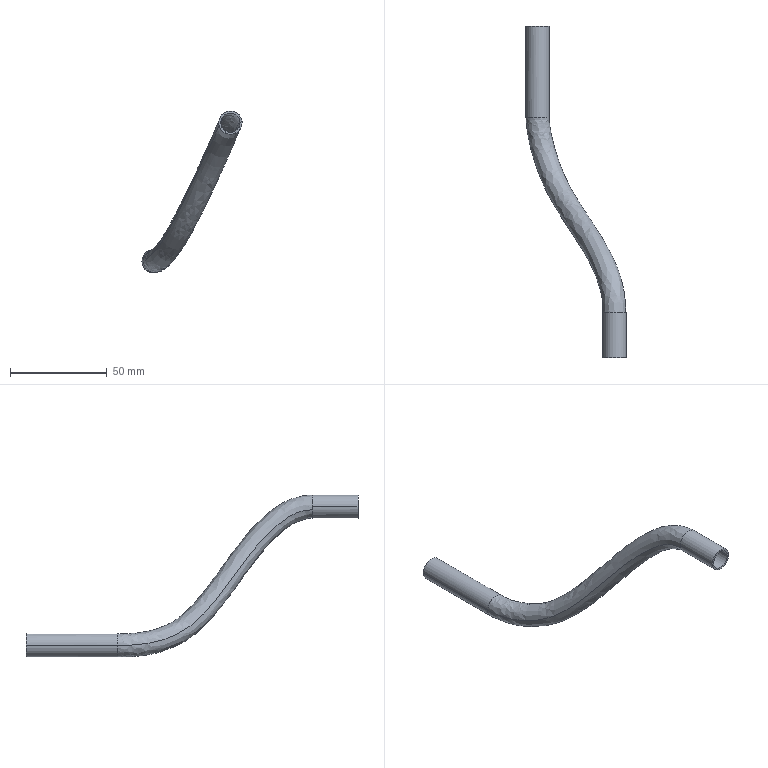Part | SolidWorks | features 3DProfileFeature 2, Sweep 1 | 1 solid | 14 faces | box 51.691 x 171.416 x 83.578 mm | volume 7159 mm3 | cylinder 8 | spline 4 | plane 2 | commonest cylinder face diameters 10 x4 12 x4